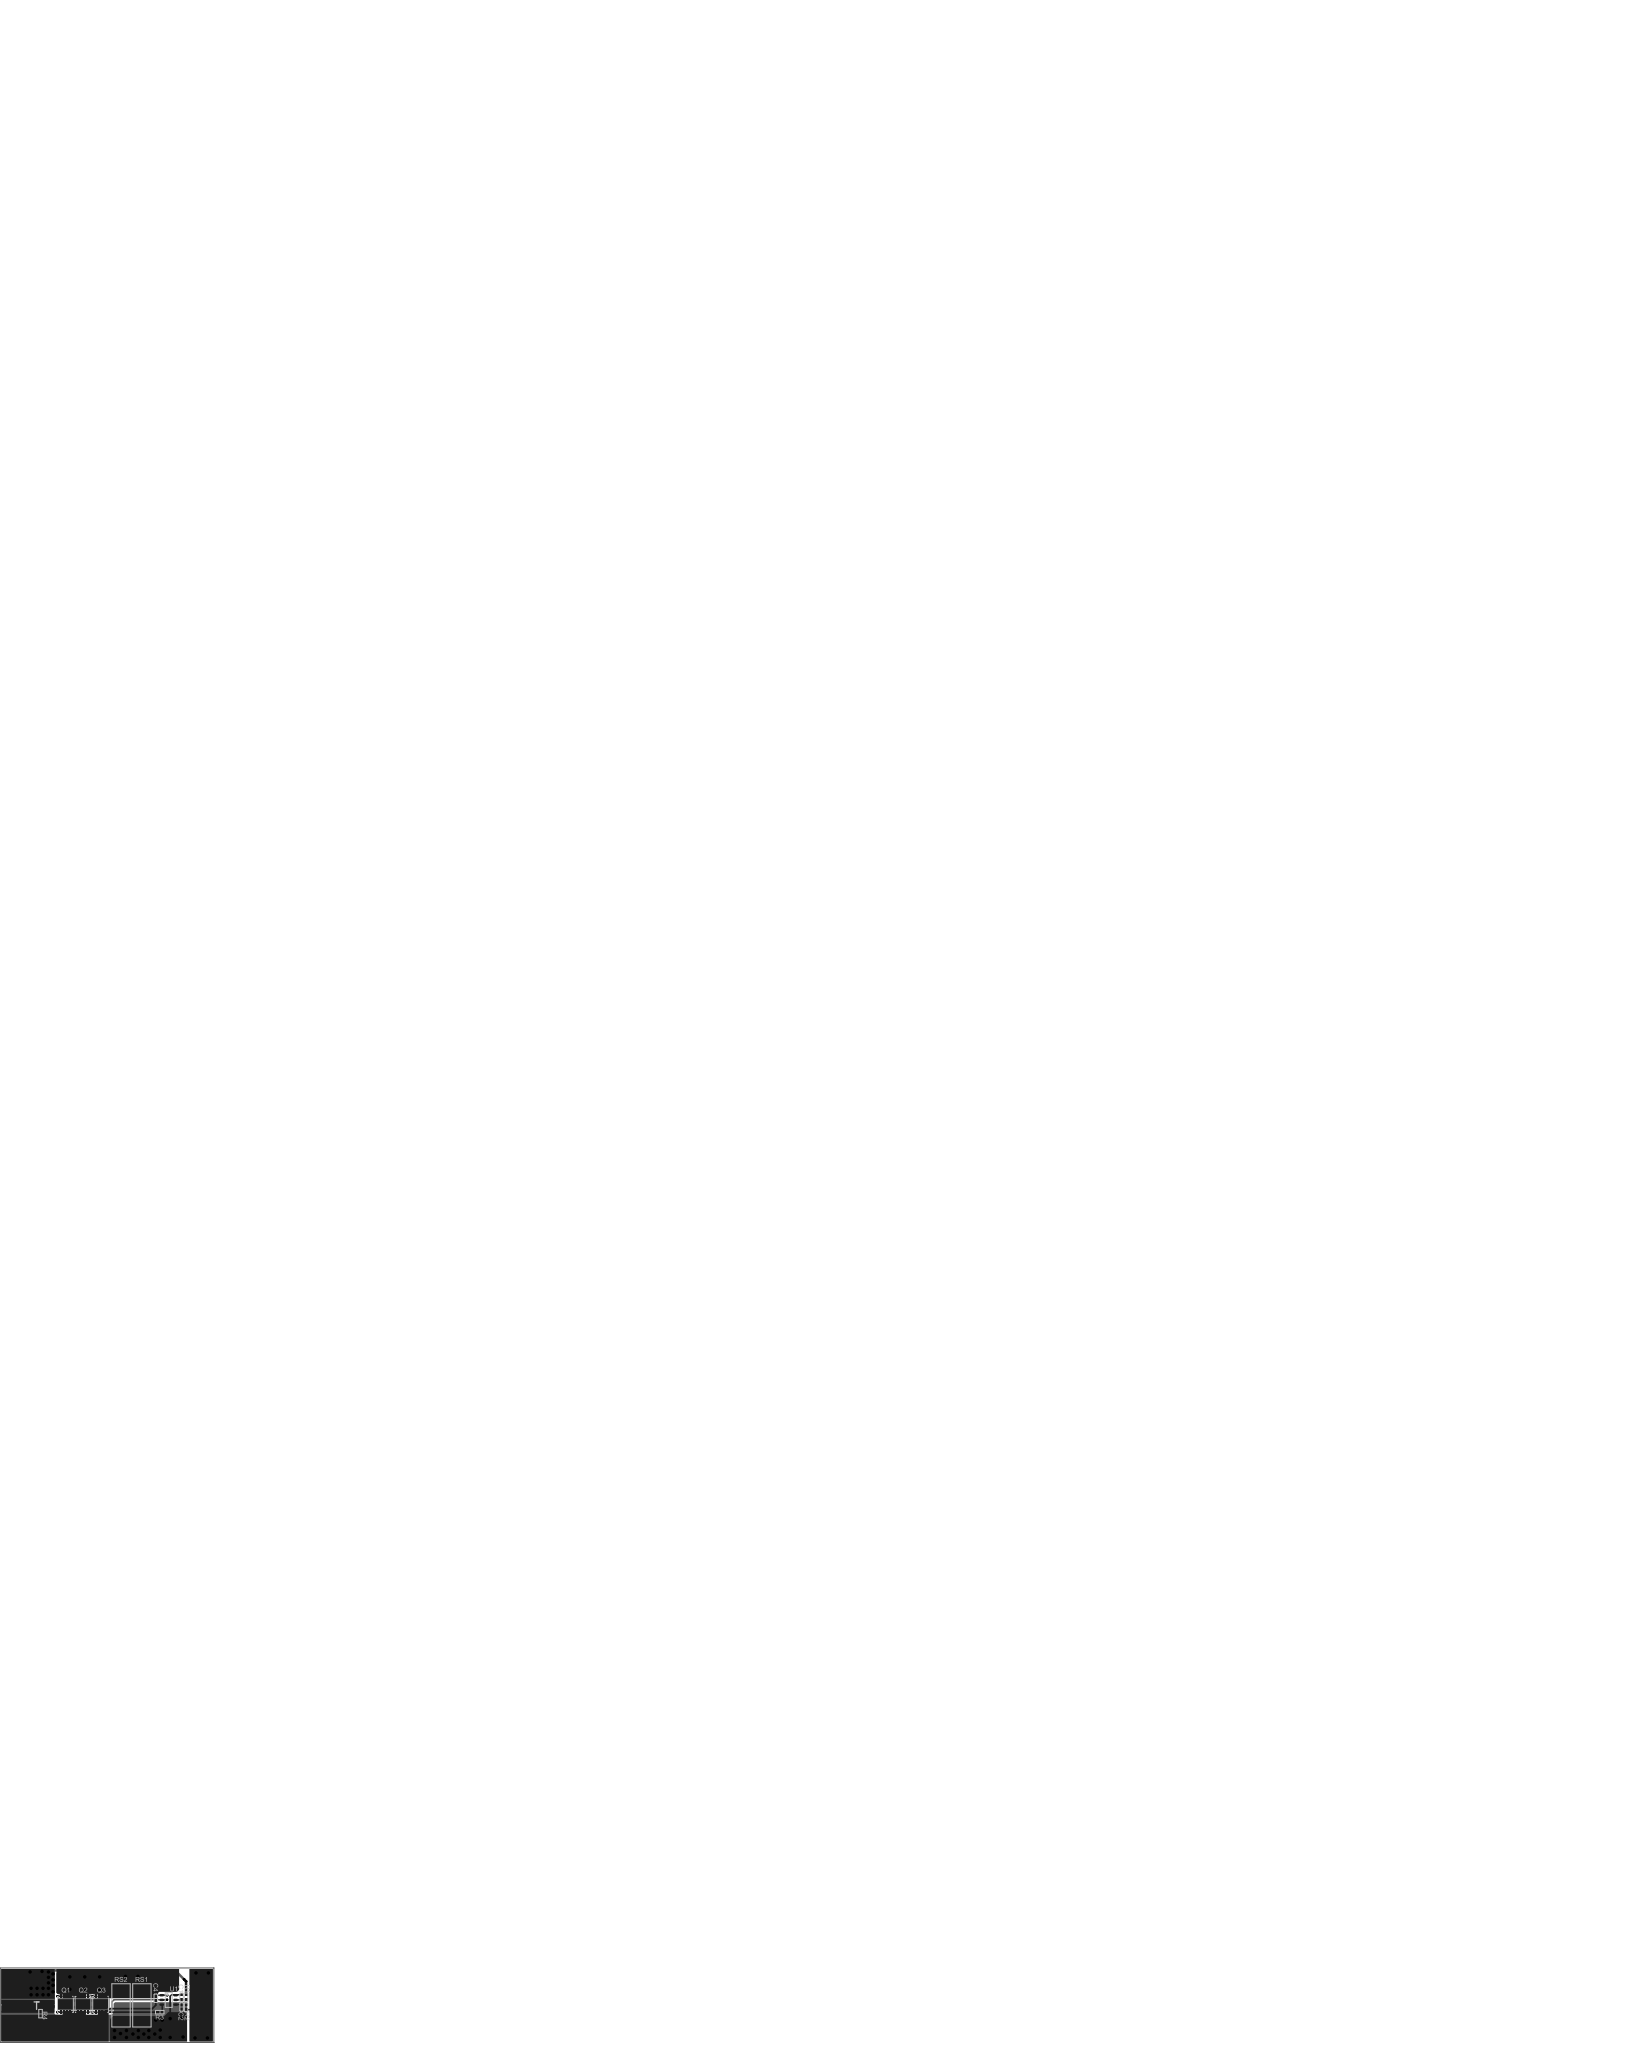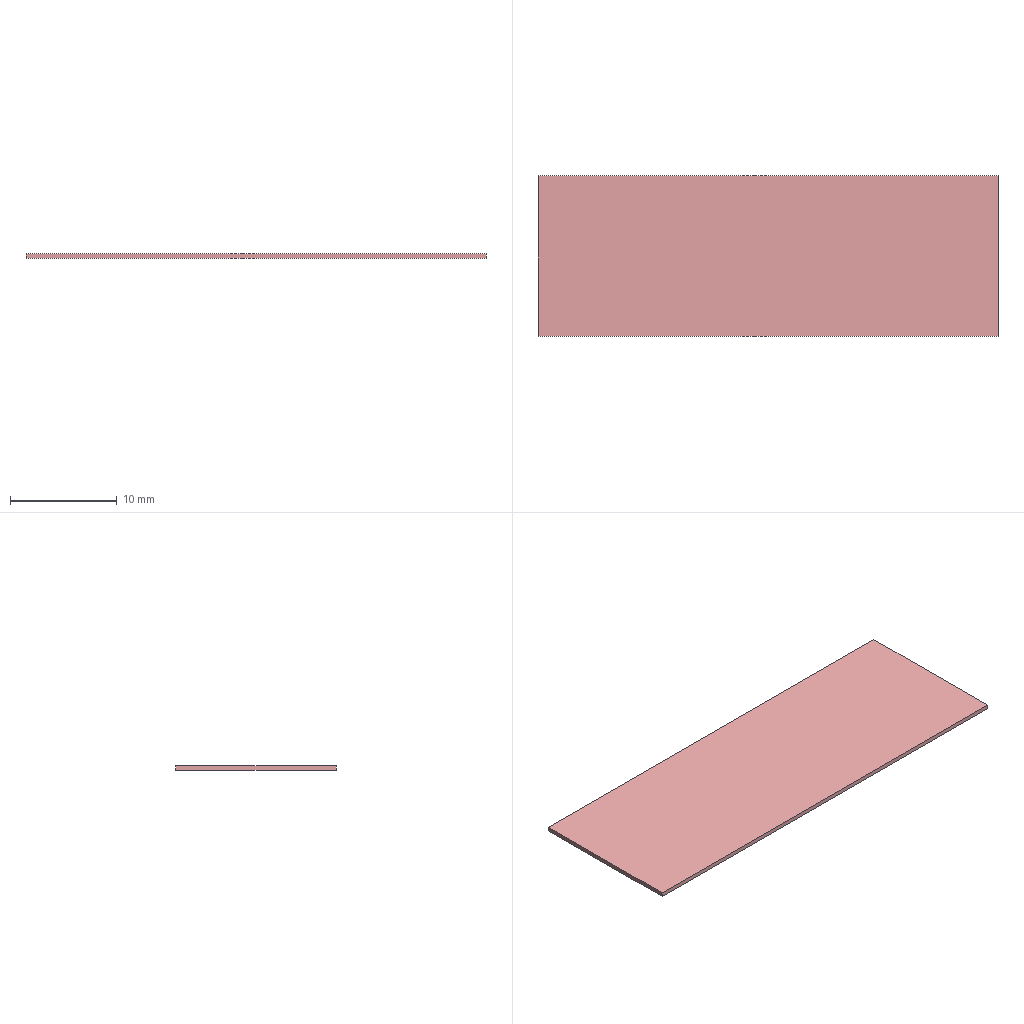Circuit board layout | Altium Designer | box 43 x 15 x 0.4 mm
Layer stack:
# Altium Designer layer stack of  (unit mm; dielectric type: 0 none, 1 core, 2 prepreg, 3 surface material)
index,name,kind,layer,copper_thickness_mm,dielectric_type,dielectric_thickness_mm,dielectric_material,dielectric_constant
0,Top Paste,other,,,,,,
1,Top Overlay,other,,,,,,
2,Top Solder,dielectric,,,3,0.0102,Solder Resist,3.5
3,Top Layer,copper,Top Layer,0.0356,,,,
4,Dielectric 1,dielectric,,,0,0.32,FR-4,4.8
5,Bottom Layer,copper,Bottom Layer,0.0356,,,,
6,Bottom Solder,dielectric,,,3,0.0102,Solder Resist,3.5
7,Bottom Overlay,other,,,,,,
8,Bottom Paste,other,,,,,,
# drill layer pairs: low layer,high layer
drill_pair,Top Layer,Bottom Layer
Part placement:
Designator,Comment,Layer,Footprint,Center-X(mm),Center-Y(mm),Rotation
RS2,R010,TopLayer,R2512L,24.307,7.462,90
RS1,R010,TopLayer,R2512L,28.507,7.462,90
T,Pad,TopLayer,Pad10X8mm,3.8,7.497,270
C4,0.1uF,TopLayer,C0402A,31.3,8.9,90
R4,10K,TopLayer,R0402A,8.1,5.8,90
Q3,N MOS,TopLayer,DFN3*3-L8(2N),20.207,7.662,180
Q2,N MOS,TopLayer,DFN3*3-L8(2N),16.657,7.662,0
Q1,N MOS,TopLayer,DFN3*3-L8(2N),13.107,7.662,180
U1,CM1020*,TopLayer,SOT23-6A,33.907,8.562,0
R3,2K,TopLayer,R0402A,32.1,6.1,0
R2,470R,TopLayer,R0402A,37.4,7.1,90
R1,470R,TopLayer,R0402A,37.4,9.1,270
C2,0.1uF,TopLayer,C0402A,36.5,7.137,90
C1,0.1uF,TopLayer,C0402A,36.5,9.1,270
BM,Pad,BottomLayer,Pad10X8mm,40.75,7.497,90
B-,Pad,BottomLayer,Pad10X8mm,2.75,3.247,270
B+,Pad,BottomLayer,Pad10X8mm,2.75,11.747,90
Pad and via stacks:
# Altium Designer via and pad stacks of  (unit mm). Each distinct definition once, with the count of objects using it.
# via: kind,start_layer,end_layer,hole_mm,diameter_mm,mode(0 simple;1 top-mid-bottom;2 full stack),diameter_per_layer,count,example_net
# pad: kind,layer,hole_mm,hole_type(0 round;1 square;2 slot),plating,top_size,top_shape(1 round;2 rect;3 octagon;9 rounded rect),mid_size,bottom_size,mode,footprint,size_per_layer,count,example
pad,Top Layer,0,0,plated,1x1,1,1x1,1x1,0,,,3,3
pad,Top Layer,0,0,plated,2x3.2,2,2x3.2,2x3.2,0,R2512L,,4,RS1.2
pad,Top Layer,0,0,plated,2.4x1.6,2,2.4x1.6,2.4x1.6,0,DFN3*3-L8(2N),,3,Q1.9
pad,Top Layer,0,0,plated,0.4x0.65,2,0.4x0.65,0.4x0.65,0,DFN3*3-L8(2N),,24,Q1.5
pad,Top Layer,0,0,plated,1.6x3,1,1.6x3,1.6x3,0,,,2,4
pad,Top Layer,0,2,plated,1.6x3,1,1.6x3,1.6x3,0,Pad10X8mm,,1,T.1
pad,Top Layer,0,0,plated,1x0.5,1,1x0.5,1x0.5,0,SOT23-6A,,6,U1.1
pad,Top Layer,0,0,plated,0.5x0.5,2,0.5x0.5,0.5x0.5,0,R0402A,,8,R1.1
pad,Top Layer,0,0,plated,0.5x0.5,2,0.5x0.5,0.5x0.5,0,C0402A,,6,C2.2
pad,Top Layer,0,0,plated,2x2,1,2x2,2x2,0,,,5,2
pad,Bottom Layer,0,0,plated,2x2,1,2x2,2x2,0,,,3,2
pad,Bottom Layer,0,2,plated,6x5,2,6x5,6x5,0,Pad10X8mm,,2,B-.1
pad,Bottom Layer,0,2,plated,5x4,2,5x4,5x4,0,Pad10X8mm,,1,BM.1
via,Top Layer,Bottom Layer,0.5,0.7,0,,49,B-
via,Top Layer,Bottom Layer,0.3048,0.508,0,,12,B+
Copper pours:
name,layer,net,type(0 solid;1 hatched;2 none)
NONET_L02_P-001,Bottom Layer,B-,0
NONET_L02_P-001,Bottom Layer,D,0
NONET_L02_P-001,Bottom Layer,NetC4_2,0
NONET_L02_P-001,Bottom Layer,B+,0
NONET_L02_P-001,Bottom Layer,BM,0
NONET_L02_P-001,Top Layer,D,0
NONET_L02_P-001,Top Layer,B-,0
NONET_L02_P-001,Top Layer,B+,0
NONET_L02_P-001,Top Layer,BM,0
NONET_L02_P-001,Top Layer,T,0
NONET_L02_P-001,Top Layer,P-,0
NONET_L02_P-001,Top Layer,NetC4_2,0
Design rules, without the lines most boards share:
# Altium Designer design rules of  (exported by Altium Designer, unit mm)
# columns: name | kind | enabled | priority | scope1 | scope2 | descriptor | typed fields (field=value)
NetAntennae | 56 | enabled | 1 | All | All | Net Antennae (Tolerance=0mm) (All) |
SilkToSilkClearance | 55 | enabled | 1 | All | All | Silk to Silk (Clearance=0mm) (All),(All) |
SilkToSolderMaskClearance | 54 | enabled | 1 | IsPad | All | Silk To Solder Mask (Clearance=0mm) (IsPad),(All) |
MinimumSolderMaskSliver | 53 | enabled | 1 | All | All | Minimum Solder Mask Sliver (Gap=0.01mm) (All),(All) |
HoleToHoleClearance | 52 | enabled | 1 | All | All | Hole To Hole Clearance (Gap=0.254mm) (All),(All) | gap=0.254
DiffPairsRouting | 51 | enabled | 1 | All | All | Differential Pairs Uncoupled Length using the Gap Constraints (Min=0.254mm) (Max=0.254mm) (Prefered=0.254mm)  and Width Constraints (Min=0.381mm) (Max=0.381mm) (Prefered=0.381mm) (All) |
HoleSize | 42 | enabled | 1 | All | All | Hole Size Constraint (Min=0.025mm) (Max=2.54mm) (All) |
Height | 50 | enabled | 1 | All | All | Height Constraint (Min=0mm) (Max=25.4mm) (Prefered=12.7mm) (All) | min_height=0 max_height=25.4
ComponentClearance | 24 | enabled | 1 | All | All | Component Clearance Constraint ( Horizontal Gap = 0.254mm, Vertical Gap = 0.254mm ) (All),(All)  | gap=0.254
SolderMaskExpansion | 13 | enabled | 1 | All | All | Solder Mask Expansion (Expansion =0.102mm) (All) | expansion=0.1016
PasteMaskExpansion | 14 | enabled | 1 | All | All | Paste Mask Expansion (Expansion =0mm) (All) | expansion=0
RoutingVias | 11 | enabled | 1 | All | All | Routing Via (MinHoleWidth=0.711mm) (MaxHoleWidth=0.711mm) (PreferredHoleWidth=0.711mm) (MinWidth=1.27mm) (MaxWidth=1.27mm) (PreferedWidth=1.27mm) (All) | via_min_hole=0.7112 via_max_hole=0.7112 via_preferred_diameter=1.27 via_preferred_hole=0.7112
RoutingCorners | 10 | enabled | 1 | All | All | Routing Corners (Style=45-Degree) (Min Setback=2.54mm) (Max Setback=2.54mm) (All) |
Width | 2 | enabled | 1 | All | All | Width Constraint (Min=0.254mm) (Max=10mm) (Preferred=0.254mm) (All) |
PolygonConnect | 20 | enabled | 1 | All | All | Polygon Connect Rule(Direct Connect )(Conductor Width=0.254mm) (Relief Angle=90 Angle) (Entries=4) (Air Gap Width=0.254mm) (All),(All) | connect_style(0=relief,1=direct,2=none)=1 relief_conductor_width=0.254 relief_entries=4
PlaneClearance | 12 | enabled | 1 | All | All | Power Plane Clearance (Clearance =0.508mm) (All) | clearance=0.508
PlaneConnect | 6 | enabled | 1 | All | All | Power Plane Connect Rule(Relief Connect )(Expansion=0.508mm) (Conductor Width=0.254mm) (Air Gap=0.254mm) (Entries=4) (All) | relief_conductor_width=0.254 relief_entries=4 relief_expansion=0.508
Clearance | 0 | enabled | 1 | All | All | Clearance Constraint (Gap=0.2mm) (All),(All) | gap=0.2